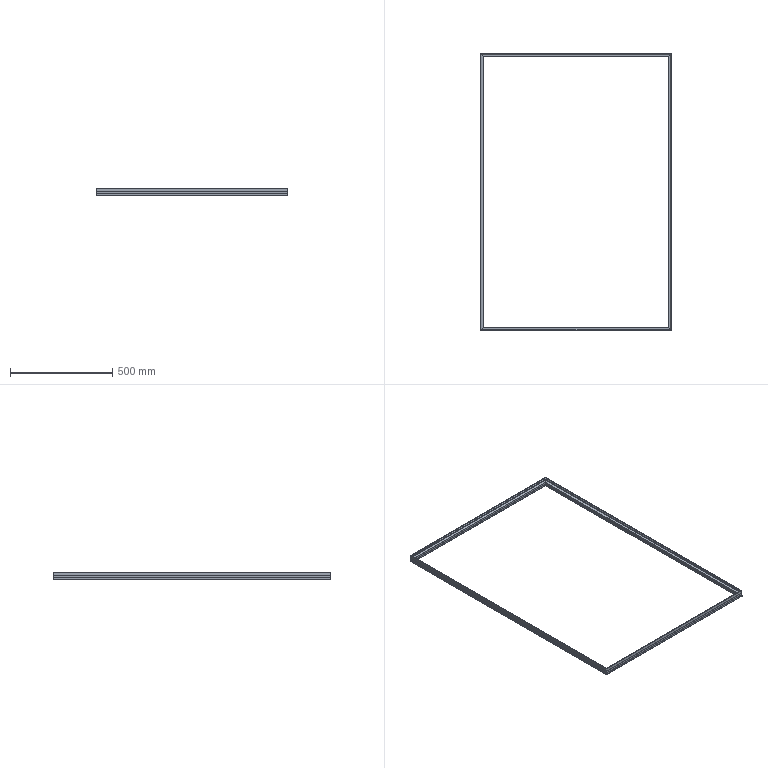Part | SolidWorks | features WeldMemberFeat 1, WeldmentFeature 1 | 4 solids | 96 faces | box 940 x 1360 x 35 mm | volume 431109 mm3 | plane 96